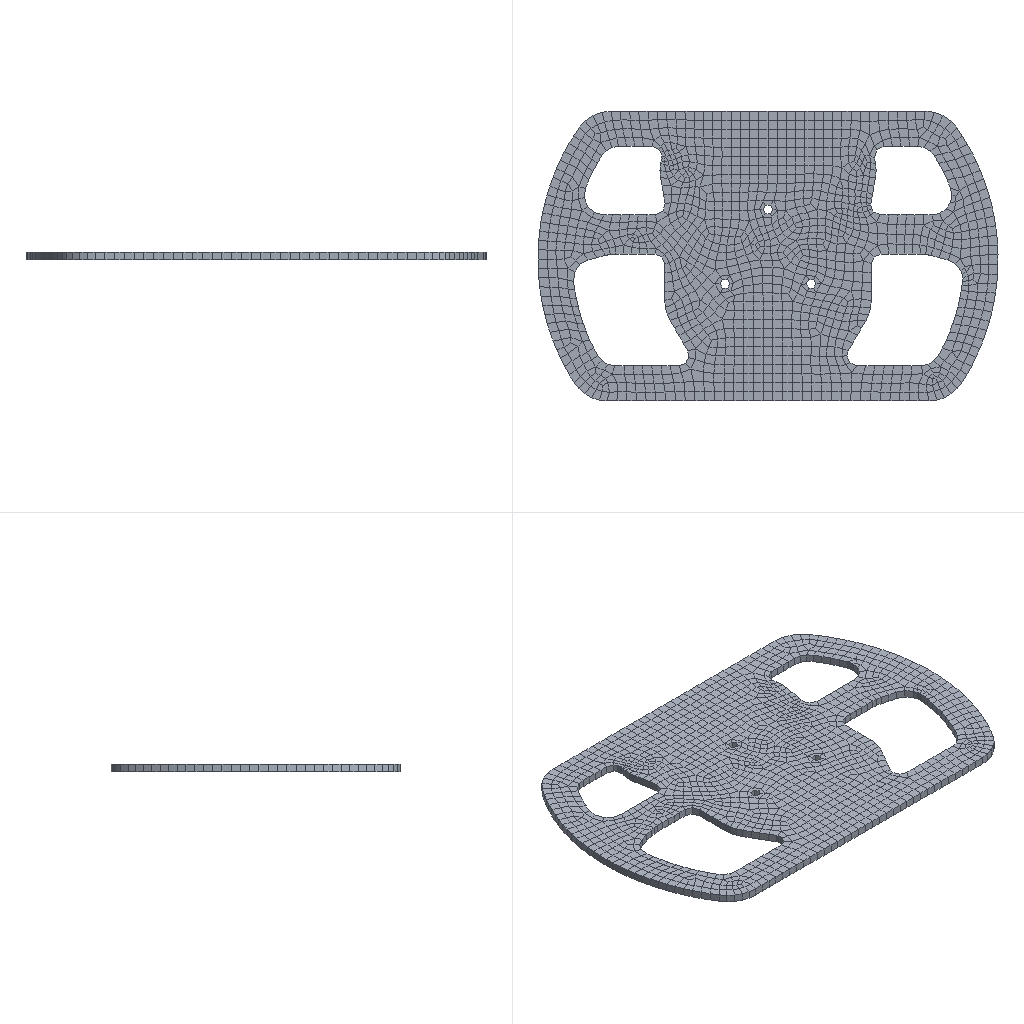Simulation study | ansys workbench
Notes in the study folder:
"Mn"= 1.5'法面模数
"Alpha"= 20'压力角
"Hax"= 1'齿顶高系数
"Cx"= 0.25'顶隙系数
"Ha"= "Hax" * "Mn"'齿顶高
"Hf"= ( "Hax" + "Cx" ) * "Mn"'齿根高
"F"= 0.38 * "Mn"'圆角
"P"=Pi*"Mt"'齿距
"Beta"= 15'螺旋角
 "Mt"="Mn" / cos ( "Beta" )'端面模数
Notes in the study folder:
"Mn"= 1.5'法面模数

"Z"= 17'齿数

"Alpha"= 20'压力角

"Beta"= 15'螺旋角

"Hax"= 1'齿顶高系数

"Cx"= 0.25'顶隙系数

"Mt"= "Mn" / cos ( "Beta" )'端面模数

"Ha"= "Hax" * "Mn"'齿顶高

"Hf"= ( "Hax" + "Cx" ) * "Mn"'齿根高

"D"= "Mt" * "Z"'分度圆直径

"Da"= "D" + 2 * "Ha"'齿顶圆直径

"Db"= "D" * cos ( "Alpha" )'齿基圆直径

"Df"= "D" - 2 * "Hf"'齿根圆直径

"r"= "D" / 2'分度圆半径

"ra"= "Da" / 2'齿顶圆半径

"rb"= "Db" / 2'齿基圆半径

"rf"= "Df" / 2'齿根圆半径

"Offset"= ( Pi * "Mt" ) / ( 4 * "r" ) - tan ( arccos ( "rb" / "r" ) ) + ( arccos ( "rb" / "r" ) * Pi ) / 180'渐开线偏移角度

"t1"= 0'渐开线起点值

"t2"= tan ( arccos ( "rb" / "ra" ) )'渐开线终点值

"Start_angle"= pI / 2 - ( tan ( arccos ( "rb" / "ra" ) ) - ( arccos ( "rb" / "ra" ) * Pi ) / 180 + "Offset" )'螺旋线起点角度

"P"= ( Pi * "Mt" * ( "Z" + 2 * cos ( "Beta" ) ) ) / tan ( "Beta" )'螺旋线螺距

"H"= 18'齿厚

"F"= 0.38 * "Mn"'圆角
Set-up summary:
category,name,step,type,value,unit,region
solver,ansys_workbench
units,mm-N-s-tonne (MPa),,stated,"/units,MPA"
analysis,LS1,,static
load_step,LS1,LS1,static,nsubst=1; time=1
mesh,nodes,,,10496
mesh,elements,,,2774
element_type,SOLID186,,,1387
element_type,SURF154,,,1387
material,Structural Steel,,E,200000,tonne s^-2 mm^-1
material,Structural Steel,,nu,0.3
material,Structural Steel,,density,7.85e-09,tonne mm^-3
material,Structural Steel,,conductivity,60.5,tonne mm s^-3 C^-1
material,Structural Steel,,specific_heat,4.34e+08,mm^2 s^-2 C^-1
material,Structural Steel,,cte,1.2e-05,C^-1
material,Structural Steel,,permeability,10000
material,Structural Steel,,resistivity,0.00017,ohm mm
load,Define Force Using Surface Effect Elements,LS1,surface-effect pres face 3,-0.0203,,SURF154 #2
bc,Fixed Supports,model,fixed,[dofs=ALL],,_FIXEDSU
named_set,_FIXEDSU,,node,90
Ansys APDL input file, long lists of numbers shortened:
/batch
/config,noeldb,1     ! force off writing results to database
*get,_wallstrt,active,,time,wall
! ANSYS input file written by Workbench version 2022 R1
! File used for geometry attach:
/title,wbnew--____ (A5)
! ****** Begin Custom Load Command Snippet ******
/COM, ACT Extensions:
/COM,     LSDYNA, 2021.1
/COM,
! ****** End   Custom Load Command Snippet ******
*DIM,_wb_ProjectScratch_dir,string,248
_wb_ProjectScratch_dir(1) = ''
*DIM,_wb_SolverFiles_dir,string,248
_wb_SolverFiles_dir(1) = ''
*DIM,_wb_userfiles_dir,string,248
_wb_userfiles_dir(1) = ''
/com,--- Data in consistent NMM units. See Solving Units in the help system for more information.
/units,MPA
/nopr
/wb,file,start              !  signify a WB generated input file
/prep7
! Turn off shape checking because checks already performed inside WB mesher.
! See help system for more information.
SHPP,OFF,,NOWARN
/nolist
etcon,set             ! allow ANSYS to choose best KEYOP's for 180x elements, resets any applicable keyopt to MAPDL defaults
/com,*********** Nodes for the whole assembly ***********
nblock,3,,11545
(1i9,3e20.9e3)
        1     5.029680982E+01     2.881305579E+01     4.000000000E+00
! (10495 more lines like these left out)
-1
/wb,elem,start            !  set before creation of elements
/com,*********** Elements for Body 1 "_____-FreeParts|__-__2" ***********
et,1,186
keyo,1,2,1          ! set full integration on SOLID186
eblock,19,solid,,1387
(19i9)
        1        1        1        1        0        0        0        0       20        0        1      334      335      851      822     2099     2098     1582     1611
! (2773 more lines like these left out)
-1
/wb,elem,end               !  done creating elements
/com,*********** Send User Defined Coordinate System(s) ***********
csys,0
toffst,273.15,  ! Temperature offset from absolute zero
/com,*********** Set Reference Temperature ***********
tref,22.
/wb,mat,start              !  starting to send materials
/com,*********** Send Materials ***********
Temperature = 'TEMP' ! Temperature
MP,DENS,1,7.85e-09,	! tonne mm^-3
MP,ALPX,1,1.2e-05,	! C^-1
MP,C,1,434000000,	! mm^2 s^-2 C^-1
MP,KXX,1,60.5,	! tonne mm s^-3 C^-1
MP,RSVX,1,0.00017,	! ohm mm
MP,EX,1,200000,	! tonne s^-2 mm^-1
MP,NUXY,1,0.3,
MP,MURX,1,10000,
/wb,mat,end                !  done sending materials
!************************* Model Summary ********************
!_____-FreeParts|__-__2,	结构钢,	matid,	1
!************************* End Model Summary ********************
! get the diagonal of the bounding box. Needed later for other things
*get,_xmin,node,,mnloc,x
*get,_ymin,node,,mnloc,y
*get,_zmin,node,,mnloc,z
*get,_xmax,node,,mxloc,x
*get,_ymax,node,,mxloc,y
*get,_zmax,node,,mxloc,z
_ASMDIAG=(_xmax-_xmin)*(_xmax-_xmin)+(_ymax-_ymin)*(_ymax-_ymin)+(_zmax-_zmin)*(_zmax-_zmin)
_ASMDIAG=SQRT(_ASMDIAG)
/wb,contact,start          !  starting to send contact
/wb,contact,end            !  done creating contacts
/golist
/wb,load,start             !  starting to send loads
/com,*********** Fixed Supports ***********
CMBLOCK,_FIXEDSU,NODE,       90
(8i10)
      2596      2597      2598      2599      2600      2601      2730      2731
! (11 more lines like these left out)
cmsel,s,_FIXEDSU
d,all,all
nsel,all
/com,*********** Define Force Using Surface Effect Elements ***********
local,12,0,0.,0.,0.,0.,0.,0.
csys,0
et,2,154
eblock,10,,,1387
(15i9)
     4488        2        2        2       12       75      227      847      847     3423     4074      847     3426
! (1386 more lines like these left out)
-1
esel,s,type,,2
keyop,2,2,1                ! Apply load in local coordinate system
keyop,2,7,1                ! Use original area so load is constant in large deformation
esel,all
/gst,on,on
fini
*get,_numnode,node,0,count
*get,_numelem,elem,0,count
*get, _MAXELEMNUM, elem, 0, NUM, MAX
*get, _MAXNODENUM, node, 0, NUM, MAX
*get, _MAXELEMTYPE, etyp, 0, NUM, MAX
*get, _MAXREALCONST, real, 0, NUM, MAX
/go
/wb,load,end               !  done creating loads
/com,--- Number of total nodes = %_numnode%
/com,--- Number of contact elements = 1387
/com,--- Number of spring elements = 0
/com,--- Number of bearing elements = 0
/com,--- Number of solid elements = 1387
/com,--- Number of condensed parts = 0
/com,--- Number of total elements = %_numelem%
*get,_wallbsol,active,,time,wall
/com,****************************************************************************
/com,*************************    SOLUTION       ********************************
/com,****************************************************************************
/solu
antype,0                   ! static analysis
_thickRatio=  0     ! Ratio of thick parts in the model
eqsl,sparse,,,,,1
cntr,print,1               ! print out contact info and also make no initial contact an error
dmpoption,emat,no             ! Don't combine emat file for DANSYS
dmpoption,esav,no             ! Don't combine esav file for DANSYS
nldiag,cont,iter           ! print out contact info each equilibrium iteration
rescontrol,,none                 ! Do not keep any restart files
/com,****************************************************
/com,******************* SOLVE FOR LS 1 OF 1 ****************
esel,s,type,,2
nsle
sfe,all,1,pres,1,0.
sfe,all,2,pres,1,0.
sfe,all,3,pres,1,-2.02984499157541e-002
nsel,all
esel,all
/nopr
/gopr
nsub,1,1,1
time,1.
outres,erase
outres,all,none
outres,nsol,all,
outres,rsol,all
outres,eangl,all
outres,etmp,all
outres,veng,all
outres,strs,all,
outres,epel,all,
outres,eppl,all,
outres,cont,all,
! *********** WB SOLVE COMMAND ***********
! check interactive state
*get,ANSINTER_,active,,int
*if,ANSINTER_,ne,0,then
/eof
*endif
solve
/com *************** Write FE CONNECTORS *********
CEWRITE,file,ce,,INTE
/com,****************************************************
/com,*************** FINISHED SOLVE FOR LS 1 *************
*get,_wallasol,active,,time,wall
/nopr
*get,_numnode,node,0,count
*get,_numelem,elem,0,count
*get, _MAXELEMNUM, elem, 0, NUM, MAX
*get, _MAXNODENUM, node, 0, NUM, MAX,,,INTERNAL
*get, _MAXELEMTYPE, etyp, 0, NUM, MAX
*get, _MAXREALCONST, real, 0, NUM, MAX
/gopr
/post1
xmlo,ENCODING,ISO-8859-1
xmlo,parm
/xml,parm,xml
fini
/gopr
*get,_walldone,active,,time,wall
_preptime=(_wallbsol-_wallstrt)*3600
_solvtime=(_wallasol-_wallbsol)*3600
_posttime=(_walldone-_wallasol)*3600
_totaltim=(_walldone-_wallstrt)*3600
*get,_dlbratio,active,0,solu,dlbr
*get,_combtime,active,0,solu,comb
*get,_ssmode,active,0,solu,ssmm
*get,_ndofs,active,0,solu,ndof
*get,_sol_end_time,active,0,set,time
*if,_sol_end_time,eq,1.,then
/fclean				!clean distributed files
*endif
/com,--- Total number of nodes = %_numnode%
/com,--- Total number of elements = %_numelem%
/com,--- Element load balance ratio = %_dlbratio%
/com,--- Time to combine distributed files = %_combtime%
/com,--- Sparse memory mode = %_ssmode%
/com,--- Number of DOF = %_ndofs%
/wb,file,end               ! done with WB generated input
Results summary:
result,analyses[0].index,,,1
result,analyses[0].system,,,SYS
result,analyses[0].deck,,,deck.dat
result,analyses[0].solve_status,,,completed
result,analyses[0].analysis_type,,,static
result,analyses[0].physics,,,mechanical
result,analyses[0].unit_system,,,"NMM: mm, ton, N, s, mV, mA, degC"
result,analyses[0].n_sets,,,1
result,analyses[0].load_steps[0].set,set=1,,1
result,analyses[0].load_steps[0].time_or_freq,set=1,,1
result,analyses[0].load_steps[0].max_displacement_magnitude,set=1,,0.2369
result,analyses[0].load_steps[0].max_von_mises_nodal,set=1,,71.902
result,analyses[0].load_steps[0].reaction_force_sum_xyz[1],set=1,,9.20933e-09
result,analyses[0].load_steps[0].reaction_force_sum_xyz[2],set=1,,-2.11169e-09
result,analyses[0].load_steps[0].reaction_force_sum_xyz[3],set=1,,500